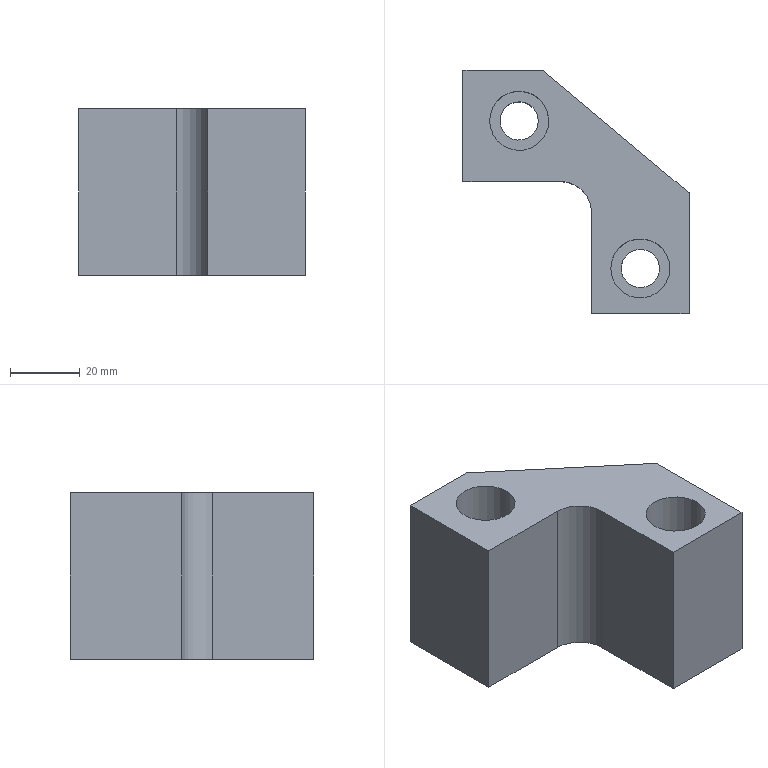Part | STEP file | gslz 2016.10.28-13_id410_x_t | 1 solid | 16 faces | box 65 x 70 x 48 mm | volume 100380 mm3 | plane 11 | cylinder 5 | commonest cylinder face diameters 11 x2 17 x2 18 x1
STEP:
#1=CARTESIAN_POINT('',(0.,0.,0.));
#2=DIRECTION('',(0.,0.,1.));
#3=DIRECTION('',(1.,0.,0.));
#4=AXIS2_PLACEMENT_3D('',#1,#2,#3);
#5=CARTESIAN_POINT('',(-792.811,143.164,0.));
#6=VERTEX_POINT('',#5);
#7=CARTESIAN_POINT('',(-792.811,108.466,0.));
#8=VERTEX_POINT('',#7);
#9=CARTESIAN_POINT('',(-792.811,119.466,0.));
#10=DIRECTION('',(0.,-1.,0.));
#11=VECTOR('',#10,1.);
#12=LINE('',#9,#11);
#13=CARTESIAN_POINT('',(-903.298,257.488,0.));
#14=DIRECTION('',(0.,0.,-1.));
#15=DIRECTION('',(-1.,0.,0.));
#16=AXIS2_PLACEMENT_3D('',#13,#14,#15);
#17=PLANE('',#16);
#18=CARTESIAN_POINT('',(-110.486,-138.022));
#19=DIRECTION('',(0.,-1.));
#20=VECTOR('',#19,1.);
#21=LINE('',#18,#20);
#22=(GEOMETRIC_REPRESENTATION_CONTEXT(2)PARAMETRIC_REPRESENTATION_CONTEXT()REPRESENTATION_CONTEXT('',''));
#23=DEFINITIONAL_REPRESENTATION('',(#21),#22);
#24=PCURVE('',#17,#23);
#25=CARTESIAN_POINT('',(-792.811,119.466,-13.75));
#26=DIRECTION('',(1.,0.,0.));
#27=DIRECTION('',(0.,0.,-1.));
#28=AXIS2_PLACEMENT_3D('',#25,#26,#27);
#29=PLANE('',#28);
#30=CARTESIAN_POINT('',(-13.75,0.));
#31=DIRECTION('',(0.,-1.));
#32=VECTOR('',#31,1.);
#33=LINE('',#30,#32);
#34=(GEOMETRIC_REPRESENTATION_CONTEXT(2)PARAMETRIC_REPRESENTATION_CONTEXT()REPRESENTATION_CONTEXT('',''));
#35=DEFINITIONAL_REPRESENTATION('',(#33),#34);
#36=PCURVE('',#29,#35);
#37=SURFACE_CURVE('',#12,(#24,#36),.PCURVE_S1.);
#38=EDGE_CURVE('',#6,#8,#37,.T.);
#39=ORIENTED_EDGE('',*,*,#38,.F.);
#40=CARTESIAN_POINT('',(-834.883,178.466,0.));
#41=VERTEX_POINT('',#40);
#42=CARTESIAN_POINT('',(-810.301,157.839,0.));
#43=DIRECTION('',(0.766,-0.6428,0.));
#44=VECTOR('',#43,1.);
#45=LINE('',#42,#44);
#46=CARTESIAN_POINT('',(-92.997,-99.649));
#47=DIRECTION('',(-0.766,-0.6428));
#48=VECTOR('',#47,1.);
#49=LINE('',#46,#48);
#50=(GEOMETRIC_REPRESENTATION_CONTEXT(2)PARAMETRIC_REPRESENTATION_CONTEXT()REPRESENTATION_CONTEXT('',''));
#51=DEFINITIONAL_REPRESENTATION('',(#49),#50);
#52=PCURVE('',#17,#51);
#53=CARTESIAN_POINT('',(-810.301,157.839,-13.75));
#54=DIRECTION('',(0.6428,0.766,0.));
#55=DIRECTION('',(0.,0.,1.));
#56=AXIS2_PLACEMENT_3D('',#53,#54,#55);
#57=PLANE('',#56);
#58=CARTESIAN_POINT('',(13.75,0.));
#59=DIRECTION('',(0.,1.));
#60=VECTOR('',#59,1.);
#61=LINE('',#58,#60);
#62=(GEOMETRIC_REPRESENTATION_CONTEXT(2)PARAMETRIC_REPRESENTATION_CONTEXT()REPRESENTATION_CONTEXT('',''));
#63=DEFINITIONAL_REPRESENTATION('',(#61),#62);
#64=PCURVE('',#57,#63);
#65=SURFACE_CURVE('',#45,(#52,#64),.PCURVE_S1.);
#66=EDGE_CURVE('',#41,#6,#65,.T.);
#67=ORIENTED_EDGE('',*,*,#66,.F.);
#68=CARTESIAN_POINT('',(-857.811,178.466,0.));
#69=VERTEX_POINT('',#68);
#70=CARTESIAN_POINT('',(-832.811,178.466,0.));
#71=DIRECTION('',(1.,0.,0.));
#72=VECTOR('',#71,1.);
#73=LINE('',#70,#72);
#74=CARTESIAN_POINT('',(-70.486,-79.022));
#75=DIRECTION('',(-1.,0.));
#76=VECTOR('',#75,1.);
#77=LINE('',#74,#76);
#78=(GEOMETRIC_REPRESENTATION_CONTEXT(2)PARAMETRIC_REPRESENTATION_CONTEXT()REPRESENTATION_CONTEXT('',''));
#79=DEFINITIONAL_REPRESENTATION('',(#77),#78);
#80=PCURVE('',#17,#79);
#81=CARTESIAN_POINT('',(-832.811,178.466,-13.75));
#82=DIRECTION('',(0.,-1.,0.));
#83=DIRECTION('',(0.,0.,-1.));
#84=AXIS2_PLACEMENT_3D('',#81,#82,#83);
#85=PLANE('',#84);
#86=CARTESIAN_POINT('',(-13.75,0.));
#87=DIRECTION('',(0.,1.));
#88=VECTOR('',#87,1.);
#89=LINE('',#86,#88);
#90=(GEOMETRIC_REPRESENTATION_CONTEXT(2)PARAMETRIC_REPRESENTATION_CONTEXT()REPRESENTATION_CONTEXT('',''));
#91=DEFINITIONAL_REPRESENTATION('',(#89),#90);
#92=PCURVE('',#85,#91);
#93=SURFACE_CURVE('',#73,(#80,#92),.PCURVE_S1.);
#94=EDGE_CURVE('',#69,#41,#93,.T.);
#95=ORIENTED_EDGE('',*,*,#94,.F.);
#96=CARTESIAN_POINT('',(-857.811,146.466,0.));
#97=VERTEX_POINT('',#96);
#98=CARTESIAN_POINT('',(-857.811,257.488,0.));
#99=DIRECTION('',(0.,-1.,0.));
#100=VECTOR('',#99,1.);
#101=LINE('',#98,#100);
#102=CARTESIAN_POINT('',(-45.486,0.));
#103=DIRECTION('',(0.,-1.));
#104=VECTOR('',#103,1.);
#105=LINE('',#102,#104);
#106=(GEOMETRIC_REPRESENTATION_CONTEXT(2)PARAMETRIC_REPRESENTATION_CONTEXT()REPRESENTATION_CONTEXT('',''));
#107=DEFINITIONAL_REPRESENTATION('',(#105),#106);
#108=PCURVE('',#17,#107);
#109=CARTESIAN_POINT('',(-857.811,119.466,-13.75));
#110=DIRECTION('',(1.,0.,0.));
#111=DIRECTION('',(0.,0.,-1.));
#112=AXIS2_PLACEMENT_3D('',#109,#110,#111);
#113=PLANE('',#112);
#114=CARTESIAN_POINT('',(-13.75,138.022));
#115=DIRECTION('',(0.,-1.));
#116=VECTOR('',#115,1.);
#117=LINE('',#114,#116);
#118=(GEOMETRIC_REPRESENTATION_CONTEXT(2)PARAMETRIC_REPRESENTATION_CONTEXT()REPRESENTATION_CONTEXT('',''));
#119=DEFINITIONAL_REPRESENTATION('',(#117),#118);
#120=PCURVE('',#113,#119);
#121=SURFACE_CURVE('',#101,(#108,#120),.PCURVE_S1.);
#122=EDGE_CURVE('',#69,#97,#121,.T.);
#123=ORIENTED_EDGE('',*,*,#122,.T.);
#124=CARTESIAN_POINT('',(-829.811,146.466,0.));
#125=VERTEX_POINT('',#124);
#126=CARTESIAN_POINT('',(-832.811,146.466,0.));
#127=DIRECTION('',(-1.,0.,0.));
#128=VECTOR('',#127,1.);
#129=LINE('',#126,#128);
#130=CARTESIAN_POINT('',(-70.486,-111.022));
#131=DIRECTION('',(1.,0.));
#132=VECTOR('',#131,1.);
#133=LINE('',#130,#132);
#134=(GEOMETRIC_REPRESENTATION_CONTEXT(2)PARAMETRIC_REPRESENTATION_CONTEXT()REPRESENTATION_CONTEXT('',''));
#135=DEFINITIONAL_REPRESENTATION('',(#133),#134);
#136=PCURVE('',#17,#135);
#137=CARTESIAN_POINT('',(-832.811,146.466,-13.75));
#138=DIRECTION('',(0.,-1.,0.));
#139=DIRECTION('',(0.,0.,-1.));
#140=AXIS2_PLACEMENT_3D('',#137,#138,#139);
#141=PLANE('',#140);
#142=CARTESIAN_POINT('',(-13.75,0.));
#143=DIRECTION('',(0.,-1.));
#144=VECTOR('',#143,1.);
#145=LINE('',#142,#144);
#146=(GEOMETRIC_REPRESENTATION_CONTEXT(2)PARAMETRIC_REPRESENTATION_CONTEXT()REPRESENTATION_CONTEXT('',''));
#147=DEFINITIONAL_REPRESENTATION('',(#145),#146);
#148=PCURVE('',#141,#147);
#149=SURFACE_CURVE('',#129,(#136,#148),.PCURVE_S1.);
#150=EDGE_CURVE('',#125,#97,#149,.T.);
#151=ORIENTED_EDGE('',*,*,#150,.F.);
#152=CARTESIAN_POINT('',(-820.811,137.466,0.));
#153=VERTEX_POINT('',#152);
#154=CARTESIAN_POINT('',(-829.811,137.466,0.));
#155=DIRECTION('',(0.,0.,-1.));
#156=DIRECTION('',(-1.,0.,0.));
#157=AXIS2_PLACEMENT_3D('',#154,#155,#156);
#158=CIRCLE('',#157,9.);
#159=CARTESIAN_POINT('',(-73.486,-120.022));
#160=DIRECTION('',(1.,0.));
#161=AXIS2_PLACEMENT_2D('',#159,#160);
#162=CIRCLE('',#161,9.);
#163=(GEOMETRIC_REPRESENTATION_CONTEXT(2)PARAMETRIC_REPRESENTATION_CONTEXT()REPRESENTATION_CONTEXT('',''));
#164=DEFINITIONAL_REPRESENTATION('',(#162),#163);
#165=PCURVE('',#17,#164);
#166=CARTESIAN_POINT('',(-829.811,137.466,-13.75));
#167=DIRECTION('',(0.,0.,1.));
#168=DIRECTION('',(1.,0.,0.));
#169=AXIS2_PLACEMENT_3D('',#166,#167,#168);
#170=CYLINDRICAL_SURFACE('',#169,9.);
#171=CARTESIAN_POINT('',(3.142,13.75));
#172=DIRECTION('',(-1.,0.));
#173=VECTOR('',#172,1.);
#174=LINE('',#171,#173);
#175=(GEOMETRIC_REPRESENTATION_CONTEXT(2)PARAMETRIC_REPRESENTATION_CONTEXT()REPRESENTATION_CONTEXT('',''));
#176=DEFINITIONAL_REPRESENTATION('',(#174),#175);
#177=PCURVE('',#170,#176);
#178=SURFACE_CURVE('',#158,(#165,#177),.PCURVE_S1.);
#179=EDGE_CURVE('',#125,#153,#178,.T.);
#180=ORIENTED_EDGE('',*,*,#179,.T.);
#181=CARTESIAN_POINT('',(-820.811,108.466,0.));
#182=VERTEX_POINT('',#181);
#183=CARTESIAN_POINT('',(-820.811,121.466,0.));
#184=DIRECTION('',(0.,-1.,0.));
#185=VECTOR('',#184,1.);
#186=LINE('',#183,#185);
#187=CARTESIAN_POINT('',(-82.486,-136.022));
#188=DIRECTION('',(0.,-1.));
#189=VECTOR('',#188,1.);
#190=LINE('',#187,#189);
#191=(GEOMETRIC_REPRESENTATION_CONTEXT(2)PARAMETRIC_REPRESENTATION_CONTEXT()REPRESENTATION_CONTEXT('',''));
#192=DEFINITIONAL_REPRESENTATION('',(#190),#191);
#193=PCURVE('',#17,#192);
#194=CARTESIAN_POINT('',(-820.811,121.466,-13.75));
#195=DIRECTION('',(1.,0.,0.));
#196=DIRECTION('',(0.,0.,-1.));
#197=AXIS2_PLACEMENT_3D('',#194,#195,#196);
#198=PLANE('',#197);
#199=CARTESIAN_POINT('',(-13.75,0.));
#200=DIRECTION('',(0.,-1.));
#201=VECTOR('',#200,1.);
#202=LINE('',#199,#201);
#203=(GEOMETRIC_REPRESENTATION_CONTEXT(2)PARAMETRIC_REPRESENTATION_CONTEXT()REPRESENTATION_CONTEXT('',''));
#204=DEFINITIONAL_REPRESENTATION('',(#202),#203);
#205=PCURVE('',#198,#204);
#206=SURFACE_CURVE('',#186,(#193,#205),.PCURVE_S1.);
#207=EDGE_CURVE('',#153,#182,#206,.T.);
#208=ORIENTED_EDGE('',*,*,#207,.T.);
#209=CARTESIAN_POINT('',(-832.811,108.466,0.));
#210=DIRECTION('',(-1.,0.,0.));
#211=VECTOR('',#210,1.);
#212=LINE('',#209,#211);
#213=CARTESIAN_POINT('',(-70.486,-149.022));
#214=DIRECTION('',(1.,0.));
#215=VECTOR('',#214,1.);
#216=LINE('',#213,#215);
#217=(GEOMETRIC_REPRESENTATION_CONTEXT(2)PARAMETRIC_REPRESENTATION_CONTEXT()REPRESENTATION_CONTEXT('',''));
#218=DEFINITIONAL_REPRESENTATION('',(#216),#217);
#219=PCURVE('',#17,#218);
#220=CARTESIAN_POINT('',(-832.811,108.466,-13.75));
#221=DIRECTION('',(0.,-1.,0.));
#222=DIRECTION('',(0.,0.,-1.));
#223=AXIS2_PLACEMENT_3D('',#220,#221,#222);
#224=PLANE('',#223);
#225=CARTESIAN_POINT('',(-13.75,0.));
#226=DIRECTION('',(0.,-1.));
#227=VECTOR('',#226,1.);
#228=LINE('',#225,#227);
#229=(GEOMETRIC_REPRESENTATION_CONTEXT(2)PARAMETRIC_REPRESENTATION_CONTEXT()REPRESENTATION_CONTEXT('',''));
#230=DEFINITIONAL_REPRESENTATION('',(#228),#229);
#231=PCURVE('',#224,#230);
#232=SURFACE_CURVE('',#212,(#219,#231),.PCURVE_S1.);
#233=EDGE_CURVE('',#8,#182,#232,.T.);
#234=ORIENTED_EDGE('',*,*,#233,.F.);
#235=EDGE_LOOP('',(#39,#67,#95,#123,#151,#180,#208,#234));
#236=FACE_BOUND('',#235,.T.);
#237=CARTESIAN_POINT('',(-815.311,121.466,0.));
#238=VERTEX_POINT('',#237);
#239=CARTESIAN_POINT('',(-806.811,121.466,0.));
#240=DIRECTION('',(0.,0.,-1.));
#241=DIRECTION('',(-1.,0.,0.));
#242=AXIS2_PLACEMENT_3D('',#239,#240,#241);
#243=CIRCLE('',#242,8.5);
#244=CARTESIAN_POINT('',(-96.486,-136.022));
#245=DIRECTION('',(1.,0.));
#246=AXIS2_PLACEMENT_2D('',#244,#245);
#247=CIRCLE('',#246,8.5);
#248=(GEOMETRIC_REPRESENTATION_CONTEXT(2)PARAMETRIC_REPRESENTATION_CONTEXT()REPRESENTATION_CONTEXT('',''));
#249=DEFINITIONAL_REPRESENTATION('',(#247),#248);
#250=PCURVE('',#17,#249);
#251=CARTESIAN_POINT('',(-806.811,121.466,0.));
#252=DIRECTION('',(0.,0.,-1.));
#253=DIRECTION('',(-1.,0.,0.));
#254=AXIS2_PLACEMENT_3D('',#251,#252,#253);
#255=CYLINDRICAL_SURFACE('',#254,8.5);
#256=CARTESIAN_POINT('',(0.,0.));
#257=DIRECTION('',(1.,0.));
#258=VECTOR('',#257,1.);
#259=LINE('',#256,#258);
#260=(GEOMETRIC_REPRESENTATION_CONTEXT(2)PARAMETRIC_REPRESENTATION_CONTEXT()REPRESENTATION_CONTEXT('',''));
#261=DEFINITIONAL_REPRESENTATION('',(#259),#260);
#262=PCURVE('',#255,#261);
#263=SURFACE_CURVE('',#243,(#250,#262),.PCURVE_S1.);
#264=EDGE_CURVE('',#238,#238,#263,.T.);
#265=ORIENTED_EDGE('',*,*,#264,.T.);
#266=EDGE_LOOP('',(#265));
#267=FACE_BOUND('',#266,.T.);
#268=CARTESIAN_POINT('',(-848.157,169.355,0.));
#269=VERTEX_POINT('',#268);
#270=CARTESIAN_POINT('',(-841.646,163.891,0.));
#271=DIRECTION('',(0.,0.,-1.));
#272=DIRECTION('',(-0.766,0.6428,0.));
#273=AXIS2_PLACEMENT_3D('',#270,#271,#272);
#274=CIRCLE('',#273,8.5);
#275=CARTESIAN_POINT('',(-61.652,-93.597));
#276=DIRECTION('',(0.766,0.6428));
#277=AXIS2_PLACEMENT_2D('',#275,#276);
#278=CIRCLE('',#277,8.5);
#279=(GEOMETRIC_REPRESENTATION_CONTEXT(2)PARAMETRIC_REPRESENTATION_CONTEXT()REPRESENTATION_CONTEXT('',''));
#280=DEFINITIONAL_REPRESENTATION('',(#278),#279);
#281=PCURVE('',#17,#280);
#282=CARTESIAN_POINT('',(-841.646,163.891,0.));
#283=DIRECTION('',(0.,0.,-1.));
#284=DIRECTION('',(-0.766,0.6428,0.));
#285=AXIS2_PLACEMENT_3D('',#282,#283,#284);
#286=CYLINDRICAL_SURFACE('',#285,8.5);
#287=CARTESIAN_POINT('',(0.,0.));
#288=DIRECTION('',(1.,0.));
#289=VECTOR('',#288,1.);
#290=LINE('',#287,#289);
#291=(GEOMETRIC_REPRESENTATION_CONTEXT(2)PARAMETRIC_REPRESENTATION_CONTEXT()REPRESENTATION_CONTEXT('',''));
#292=DEFINITIONAL_REPRESENTATION('',(#290),#291);
#293=PCURVE('',#286,#292);
#294=SURFACE_CURVE('',#274,(#281,#293),.PCURVE_S1.);
#295=EDGE_CURVE('',#269,#269,#294,.T.);
#296=ORIENTED_EDGE('',*,*,#295,.T.);
#297=EDGE_LOOP('',(#296));
#298=FACE_BOUND('',#297,.T.);
#299=ADVANCED_FACE('',(#236,#267,#298),#17,.F.);
#300=CARTESIAN_POINT('',(-820.811,108.466,-48.));
#301=VERTEX_POINT('',#300);
#302=CARTESIAN_POINT('',(-820.811,108.466,-13.75));
#303=DIRECTION('',(0.,0.,1.));
#304=VECTOR('',#303,1.);
#305=LINE('',#302,#304);
#306=CARTESIAN_POINT('',(0.,12.));
#307=DIRECTION('',(-1.,0.));
#308=VECTOR('',#307,1.);
#309=LINE('',#306,#308);
#310=(GEOMETRIC_REPRESENTATION_CONTEXT(2)PARAMETRIC_REPRESENTATION_CONTEXT()REPRESENTATION_CONTEXT('',''));
#311=DEFINITIONAL_REPRESENTATION('',(#309),#310);
#312=PCURVE('',#224,#311);
#313=CARTESIAN_POINT('',(0.,-13.));
#314=DIRECTION('',(-1.,0.));
#315=VECTOR('',#314,1.);
#316=LINE('',#313,#315);
#317=(GEOMETRIC_REPRESENTATION_CONTEXT(2)PARAMETRIC_REPRESENTATION_CONTEXT()REPRESENTATION_CONTEXT('',''));
#318=DEFINITIONAL_REPRESENTATION('',(#316),#317);
#319=PCURVE('',#198,#318);
#320=SURFACE_CURVE('',#305,(#312,#319),.PCURVE_S1.);
#321=EDGE_CURVE('',#301,#182,#320,.T.);
#322=ORIENTED_EDGE('',*,*,#321,.F.);
#323=CARTESIAN_POINT('',(-792.811,108.466,-48.));
#324=VERTEX_POINT('',#323);
#325=CARTESIAN_POINT('',(-832.811,108.466,-48.));
#326=DIRECTION('',(1.,0.,0.));
#327=VECTOR('',#326,1.);
#328=LINE('',#325,#327);
#329=CARTESIAN_POINT('',(34.25,0.));
#330=DIRECTION('',(0.,1.));
#331=VECTOR('',#330,1.);
#332=LINE('',#329,#331);
#333=(GEOMETRIC_REPRESENTATION_CONTEXT(2)PARAMETRIC_REPRESENTATION_CONTEXT()REPRESENTATION_CONTEXT('',''));
#334=DEFINITIONAL_REPRESENTATION('',(#332),#333);
#335=PCURVE('',#224,#334);
#336=CARTESIAN_POINT('',(-903.298,257.488,-48.));
#337=DIRECTION('',(0.,0.,-1.));
#338=DIRECTION('',(-1.,0.,0.));
#339=AXIS2_PLACEMENT_3D('',#336,#337,#338);
#340=PLANE('',#339);
#341=CARTESIAN_POINT('',(-70.486,-149.022));
#342=DIRECTION('',(-1.,0.));
#343=VECTOR('',#342,1.);
#344=LINE('',#341,#343);
#345=(GEOMETRIC_REPRESENTATION_CONTEXT(2)PARAMETRIC_REPRESENTATION_CONTEXT()REPRESENTATION_CONTEXT('',''));
#346=DEFINITIONAL_REPRESENTATION('',(#344),#345);
#347=PCURVE('',#340,#346);
#348=SURFACE_CURVE('',#328,(#335,#347),.PCURVE_S1.);
#349=EDGE_CURVE('',#301,#324,#348,.T.);
#350=ORIENTED_EDGE('',*,*,#349,.T.);
#351=CARTESIAN_POINT('',(-792.811,108.466,-13.75));
#352=DIRECTION('',(0.,0.,1.));
#353=VECTOR('',#352,1.);
#354=LINE('',#351,#353);
#355=CARTESIAN_POINT('',(0.,40.));
#356=DIRECTION('',(-1.,0.));
#357=VECTOR('',#356,1.);
#358=LINE('',#355,#357);
#359=(GEOMETRIC_REPRESENTATION_CONTEXT(2)PARAMETRIC_REPRESENTATION_CONTEXT()REPRESENTATION_CONTEXT('',''));
#360=DEFINITIONAL_REPRESENTATION('',(#358),#359);
#361=PCURVE('',#224,#360);
#362=CARTESIAN_POINT('',(0.,-11.));
#363=DIRECTION('',(-1.,0.));
#364=VECTOR('',#363,1.);
#365=LINE('',#362,#364);
#366=(GEOMETRIC_REPRESENTATION_CONTEXT(2)PARAMETRIC_REPRESENTATION_CONTEXT()REPRESENTATION_CONTEXT('',''));
#367=DEFINITIONAL_REPRESENTATION('',(#365),#366);
#368=PCURVE('',#29,#367);
#369=SURFACE_CURVE('',#354,(#361,#368),.PCURVE_S1.);
#370=EDGE_CURVE('',#324,#8,#369,.T.);
#371=ORIENTED_EDGE('',*,*,#370,.T.);
#372=ORIENTED_EDGE('',*,*,#233,.T.);
#373=EDGE_LOOP('',(#322,#350,#371,#372));
#374=FACE_BOUND('',#373,.T.);
#375=ADVANCED_FACE('',(#374),#224,.T.);
#376=CARTESIAN_POINT('',(-792.811,143.164,-48.));
#377=VERTEX_POINT('',#376);
#378=CARTESIAN_POINT('',(-834.883,178.466,-48.));
#379=VERTEX_POINT('',#378);
#380=CARTESIAN_POINT('',(-810.301,157.839,-48.));
#381=DIRECTION('',(-0.766,0.6428,0.));
#382=VECTOR('',#381,1.);
#383=LINE('',#380,#382);
#384=CARTESIAN_POINT('',(-92.997,-99.649));
#385=DIRECTION('',(0.766,0.6428));
#386=VECTOR('',#385,1.);
#387=LINE('',#384,#386);
#388=(GEOMETRIC_REPRESENTATION_CONTEXT(2)PARAMETRIC_REPRESENTATION_CONTEXT()REPRESENTATION_CONTEXT('',''));
#389=DEFINITIONAL_REPRESENTATION('',(#387),#388);
#390=PCURVE('',#340,#389);
#391=CARTESIAN_POINT('',(-34.25,0.));
#392=DIRECTION('',(0.,-1.));
#393=VECTOR('',#392,1.);
#394=LINE('',#391,#393);
#395=(GEOMETRIC_REPRESENTATION_CONTEXT(2)PARAMETRIC_REPRESENTATION_CONTEXT()REPRESENTATION_CONTEXT('',''));
#396=DEFINITIONAL_REPRESENTATION('',(#394),#395);
#397=PCURVE('',#57,#396);
#398=SURFACE_CURVE('',#383,(#390,#397),.PCURVE_S1.);
#399=EDGE_CURVE('',#377,#379,#398,.T.);
#400=ORIENTED_EDGE('',*,*,#399,.F.);
#401=CARTESIAN_POINT('',(-792.811,119.466,-48.));
#402=DIRECTION('',(0.,1.,0.));
#403=VECTOR('',#402,1.);
#404=LINE('',#401,#403);
#405=CARTESIAN_POINT('',(-110.486,-138.022));
#406=DIRECTION('',(0.,1.));
#407=VECTOR('',#406,1.);
#408=LINE('',#405,#407);
#409=(GEOMETRIC_REPRESENTATION_CONTEXT(2)PARAMETRIC_REPRESENTATION_CONTEXT()REPRESENTATION_CONTEXT('',''));
#410=DEFINITIONAL_REPRESENTATION('',(#408),#409);
#411=PCURVE('',#340,#410);
#412=CARTESIAN_POINT('',(34.25,0.));
#413=DIRECTION('',(0.,1.));
#414=VECTOR('',#413,1.);
#415=LINE('',#412,#414);
#416=(GEOMETRIC_REPRESENTATION_CONTEXT(2)PARAMETRIC_REPRESENTATION_CONTEXT()REPRESENTATION_CONTEXT('',''));
#417=DEFINITIONAL_REPRESENTATION('',(#415),#416);
#418=PCURVE('',#29,#417);
#419=SURFACE_CURVE('',#404,(#411,#418),.PCURVE_S1.);
#420=EDGE_CURVE('',#324,#377,#419,.T.);
#421=ORIENTED_EDGE('',*,*,#420,.F.);
#422=ORIENTED_EDGE('',*,*,#349,.F.);
#423=CARTESIAN_POINT('',(-820.811,137.466,-48.));
#424=VERTEX_POINT('',#423);
#425=CARTESIAN_POINT('',(-820.811,259.488,-48.));
#426=DIRECTION('',(0.,-1.,0.));
#427=VECTOR('',#426,1.);
#428=LINE('',#425,#427);
#429=CARTESIAN_POINT('',(-82.486,2.));
#430=DIRECTION('',(0.,-1.));
#431=VECTOR('',#430,1.);
#432=LINE('',#429,#431);
#433=(GEOMETRIC_REPRESENTATION_CONTEXT(2)PARAMETRIC_REPRESENTATION_CONTEXT()REPRESENTATION_CONTEXT('',''));
#434=DEFINITIONAL_REPRESENTATION('',(#432),#433);
#435=PCURVE('',#340,#434);
#436=CARTESIAN_POINT('',(34.25,138.022));
#437=DIRECTION('',(0.,-1.));
#438=VECTOR('',#437,1.);
#439=LINE('',#436,#438);
#440=(GEOMETRIC_REPRESENTATION_CONTEXT(2)PARAMETRIC_REPRESENTATION_CONTEXT()REPRESENTATION_CONTEXT('',''));
#441=DEFINITIONAL_REPRESENTATION('',(#439),#440);
#442=PCURVE('',#198,#441);
#443=SURFACE_CURVE('',#428,(#435,#442),.PCURVE_S1.);
#444=EDGE_CURVE('',#424,#301,#443,.T.);
#445=ORIENTED_EDGE('',*,*,#444,.F.);
#446=CARTESIAN_POINT('',(-829.811,146.466,-48.));
#447=VERTEX_POINT('',#446);
#448=CARTESIAN_POINT('',(-829.811,137.466,-48.));
#449=DIRECTION('',(0.,0.,1.));
#450=DIRECTION('',(-1.,0.,0.));
#451=AXIS2_PLACEMENT_3D('',#448,#449,#450);
#452=CIRCLE('',#451,9.);
#453=CARTESIAN_POINT('',(-64.486,-120.022));
#454=CARTESIAN_POINT('',(-64.486,-135.611));
#455=CARTESIAN_POINT('',(-77.986,-127.816));
#456=CARTESIAN_POINT('',(-91.486,-120.022));
#457=CARTESIAN_POINT('',(-77.986,-112.228));
#458=CARTESIAN_POINT('',(-64.486,-104.434));
#459=CARTESIAN_POINT('',(-64.486,-120.022));
#460=(BOUNDED_CURVE()B_SPLINE_CURVE(2,(#453,#454,#455,#456,#457,#458,#459),.UNSPECIFIED.,.T.,.F.)B_SPLINE_CURVE_WITH_KNOTS((1,2,2,2,2,1),(-2.094,0.,2.094,4.189,6.283,8.378),.UNSPECIFIED.)CURVE()GEOMETRIC_REPRESENTATION_ITEM()RATIONAL_B_SPLINE_CURVE((1.,0.5,1.,0.5,1.,0.5,1.))REPRESENTATION_ITEM(''));
#461=(GEOMETRIC_REPRESENTATION_CONTEXT(2)PARAMETRIC_REPRESENTATION_CONTEXT()REPRESENTATION_CONTEXT('',''));
#462=DEFINITIONAL_REPRESENTATION('',(#460),#461);
#463=PCURVE('',#340,#462);
#464=CARTESIAN_POINT('',(-3.142,-34.25));
#465=DIRECTION('',(1.,0.));
#466=VECTOR('',#465,1.);
#467=LINE('',#464,#466);
#468=(GEOMETRIC_REPRESENTATION_CONTEXT(2)PARAMETRIC_REPRESENTATION_CONTEXT()REPRESENTATION_CONTEXT('',''));
#469=DEFINITIONAL_REPRESENTATION('',(#467),#468);
#470=PCURVE('',#170,#469);
#471=SURFACE_CURVE('',#452,(#463,#470),.PCURVE_S1.);
#472=EDGE_CURVE('',#424,#447,#471,.T.);
#473=ORIENTED_EDGE('',*,*,#472,.T.);
#474=CARTESIAN_POINT('',(-857.811,146.466,-48.));
#475=VERTEX_POINT('',#474);
#476=CARTESIAN_POINT('',(-832.811,146.466,-48.));
#477=DIRECTION('',(1.,0.,0.));
#478=VECTOR('',#477,1.);
#479=LINE('',#476,#478);
#480=CARTESIAN_POINT('',(-70.486,-111.022));
#481=DIRECTION('',(-1.,0.));
#482=VECTOR('',#481,1.);
#483=LINE('',#480,#482);
#484=(GEOMETRIC_REPRESENTATION_CONTEXT(2)PARAMETRIC_REPRESENTATION_CONTEXT()REPRESENTATION_CONTEXT('',''));
#485=DEFINITIONAL_REPRESENTATION('',(#483),#484);
#486=PCURVE('',#340,#485);
#487=CARTESIAN_POINT('',(34.25,0.));
#488=DIRECTION('',(0.,1.));
#489=VECTOR('',#488,1.);
#490=LINE('',#487,#489);
#491=(GEOMETRIC_REPRESENTATION_CONTEXT(2)PARAMETRIC_REPRESENTATION_CONTEXT()REPRESENTATION_CONTEXT('',''));
#492=DEFINITIONAL_REPRESENTATION('',(#490),#491);
#493=PCURVE('',#141,#492);
#494=SURFACE_CURVE('',#479,(#486,#493),.PCURVE_S1.);
#495=EDGE_CURVE('',#475,#447,#494,.T.);
#496=ORIENTED_EDGE('',*,*,#495,.F.);
#497=CARTESIAN_POINT('',(-857.811,178.466,-48.));
#498=VERTEX_POINT('',#497);
#499=CARTESIAN_POINT('',(-857.811,257.488,-48.));
#500=DIRECTION('',(0.,1.,0.));
#501=VECTOR('',#500,1.);
#502=LINE('',#499,#501);
#503=CARTESIAN_POINT('',(-45.486,0.));
#504=DIRECTION('',(0.,1.));
#505=VECTOR('',#504,1.);
#506=LINE('',#503,#505);
#507=(GEOMETRIC_REPRESENTATION_CONTEXT(2)PARAMETRIC_REPRESENTATION_CONTEXT()REPRESENTATION_CONTEXT('',''));
#508=DEFINITIONAL_REPRESENTATION('',(#506),#507);
#509=PCURVE('',#340,#508);
#510=CARTESIAN_POINT('',(34.25,138.022));
#511=DIRECTION('',(0.,1.));
#512=VECTOR('',#511,1.);
#513=LINE('',#510,#512);
#514=(GEOMETRIC_REPRESENTATION_CONTEXT(2)PARAMETRIC_REPRESENTATION_CONTEXT()REPRESENTATION_CONTEXT('',''));
#515=DEFINITIONAL_REPRESENTATION('',(#513),#514);
#516=PCURVE('',#113,#515);
#517=SURFACE_CURVE('',#502,(#509,#516),.PCURVE_S1.);
#518=EDGE_CURVE('',#475,#498,#517,.T.);
#519=ORIENTED_EDGE('',*,*,#518,.T.);
#520=CARTESIAN_POINT('',(-832.811,178.466,-48.));
#521=DIRECTION('',(-1.,0.,0.));
#522=VECTOR('',#521,1.);
#523=LINE('',#520,#522);
#524=CARTESIAN_POINT('',(-70.486,-79.022));
#525=DIRECTION('',(1.,0.));
#526=VECTOR('',#525,1.);
#527=LINE('',#524,#526);
#528=(GEOMETRIC_REPRESENTATION_CONTEXT(2)PARAMETRIC_REPRESENTATION_CONTEXT()REPRESENTATION_CONTEXT('',''));
#529=DEFINITIONAL_REPRESENTATION('',(#527),#528);
#530=PCURVE('',#340,#529);
#531=CARTESIAN_POINT('',(34.25,0.));
#532=DIRECTION('',(0.,-1.));
#533=VECTOR('',#532,1.);
#534=LINE('',#531,#533);
#535=(GEOMETRIC_REPRESENTATION_CONTEXT(2)PARAMETRIC_REPRESENTATION_CONTEXT()REPRESENTATION_CONTEXT('',''));
#536=DEFINITIONAL_REPRESENTATION('',(#534),#535);
#537=PCURVE('',#85,#536);
#538=SURFACE_CURVE('',#523,(#530,#537),.PCURVE_S1.);
#539=EDGE_CURVE('',#379,#498,#538,.T.);
#540=ORIENTED_EDGE('',*,*,#539,.F.);
#541=EDGE_LOOP('',(#400,#421,#422,#445,#473,#496,#519,#540));
#542=FACE_BOUND('',#541,.T.);
#543=CARTESIAN_POINT('',(-812.311,121.466,-48.));
#544=VERTEX_POINT('',#543);
#545=CARTESIAN_POINT('',(-806.811,121.466,-48.));
#546=DIRECTION('',(0.,0.,-1.));
#547=DIRECTION('',(-1.,0.,0.));
#548=AXIS2_PLACEMENT_3D('',#545,#546,#547);
#549=CIRCLE('',#548,5.5);
#550=CARTESIAN_POINT('',(-96.486,-136.022));
#551=DIRECTION('',(1.,0.));
#552=AXIS2_PLACEMENT_2D('',#550,#551);
#553=CIRCLE('',#552,5.5);
#554=(GEOMETRIC_REPRESENTATION_CONTEXT(2)PARAMETRIC_REPRESENTATION_CONTEXT()REPRESENTATION_CONTEXT('',''));
#555=DEFINITIONAL_REPRESENTATION('',(#553),#554);
#556=PCURVE('',#340,#555);
#557=CARTESIAN_POINT('',(-806.811,121.466,-150.));
#558=DIRECTION('',(0.,0.,-1.));
#559=DIRECTION('',(-1.,0.,0.));
#560=AXIS2_PLACEMENT_3D('',#557,#558,#559);
#561=CYLINDRICAL_SURFACE('',#560,5.5);
#562=CARTESIAN_POINT('',(0.,-102.));
#563=DIRECTION('',(1.,0.));
#564=VECTOR('',#563,1.);
#565=LINE('',#562,#564);
#566=(GEOMETRIC_REPRESENTATION_CONTEXT(2)PARAMETRIC_REPRESENTATION_CONTEXT()REPRESENTATION_CONTEXT('',''));
#567=DEFINITIONAL_REPRESENTATION('',(#565),#566);
#568=PCURVE('',#561,#567);
#569=SURFACE_CURVE('',#549,(#556,#568),.PCURVE_S1.);
#570=EDGE_CURVE('',#544,#544,#569,.T.);
#571=ORIENTED_EDGE('',*,*,#570,.F.);
#572=EDGE_LOOP('',(#571));
#573=FACE_BOUND('',#572,.T.);
#574=CARTESIAN_POINT('',(-845.859,167.426,-48.));
#575=VERTEX_POINT('',#574);
#576=CARTESIAN_POINT('',(-841.646,163.891,-48.));
#577=DIRECTION('',(0.,0.,-1.));
#578=DIRECTION('',(-0.766,0.6428,0.));
#579=AXIS2_PLACEMENT_3D('',#576,#577,#578);
#580=CIRCLE('',#579,5.5);
#581=CARTESIAN_POINT('',(-61.652,-93.597));
#582=DIRECTION('',(0.766,0.6428));
#583=AXIS2_PLACEMENT_2D('',#581,#582);
#584=CIRCLE('',#583,5.5);
#585=(GEOMETRIC_REPRESENTATION_CONTEXT(2)PARAMETRIC_REPRESENTATION_CONTEXT()REPRESENTATION_CONTEXT('',''));
#586=DEFINITIONAL_REPRESENTATION('',(#584),#585);
#587=PCURVE('',#340,#586);
#588=CARTESIAN_POINT('',(-841.646,163.891,-150.));
#589=DIRECTION('',(0.,0.,-1.));
#590=DIRECTION('',(-0.766,0.6428,0.));
#591=AXIS2_PLACEMENT_3D('',#588,#589,#590);
#592=CYLINDRICAL_SURFACE('',#591,5.5);
#593=CARTESIAN_POINT('',(0.,-102.));
#594=DIRECTION('',(1.,0.));
#595=VECTOR('',#594,1.);
#596=LINE('',#593,#595);
#597=(GEOMETRIC_REPRESENTATION_CONTEXT(2)PARAMETRIC_REPRESENTATION_CONTEXT()REPRESENTATION_CONTEXT('',''));
#598=DEFINITIONAL_REPRESENTATION('',(#596),#597);
#599=PCURVE('',#592,#598);
#600=SURFACE_CURVE('',#580,(#587,#599),.PCURVE_S1.);
#601=EDGE_CURVE('',#575,#575,#600,.T.);
#602=ORIENTED_EDGE('',*,*,#601,.F.);
#603=EDGE_LOOP('',(#602));
#604=FACE_BOUND('',#603,.T.);
#605=ADVANCED_FACE('',(#542,#573,#604),#340,.T.);
#606=ORIENTED_EDGE('',*,*,#420,.T.);
#607=CARTESIAN_POINT('',(-792.811,143.164,-13.75));
#608=DIRECTION('',(0.,0.,1.));
#609=VECTOR('',#608,1.);
#610=LINE('',#607,#609);
#611=CARTESIAN_POINT('',(0.,23.698));
#612=DIRECTION('',(-1.,0.));
#613=VECTOR('',#612,1.);
#614=LINE('',#611,#613);
#615=(GEOMETRIC_REPRESENTATION_CONTEXT(2)PARAMETRIC_REPRESENTATION_CONTEXT()REPRESENTATION_CONTEXT('',''));
#616=DEFINITIONAL_REPRESENTATION('',(#614),#615);
#617=PCURVE('',#29,#616);
#618=CARTESIAN_POINT('',(0.,22.831));
#619=DIRECTION('',(1.,0.));
#620=VECTOR('',#619,1.);
#621=LINE('',#618,#620);
#622=(GEOMETRIC_REPRESENTATION_CONTEXT(2)PARAMETRIC_REPRESENTATION_CONTEXT()REPRESENTATION_CONTEXT('',''));
#623=DEFINITIONAL_REPRESENTATION('',(#621),#622);
#624=PCURVE('',#57,#623);
#625=SURFACE_CURVE('',#610,(#617,#624),.PCURVE_S1.);
#626=EDGE_CURVE('',#377,#6,#625,.T.);
#627=ORIENTED_EDGE('',*,*,#626,.T.);
#628=ORIENTED_EDGE('',*,*,#38,.T.);
#629=ORIENTED_EDGE('',*,*,#370,.F.);
#630=EDGE_LOOP('',(#606,#627,#628,#629));
#631=FACE_BOUND('',#630,.T.);
#632=ADVANCED_FACE('',(#631),#29,.T.);
#633=ORIENTED_EDGE('',*,*,#570,.F.);
#634=CARTESIAN_POINT('',(-812.311,121.466,-25.));
#635=VERTEX_POINT('',#634);
#636=CARTESIAN_POINT('',(-812.311,121.466,-25.));
#637=CARTESIAN_POINT('',(-812.311,121.466,-48.));
#638=B_SPLINE_CURVE_WITH_KNOTS('',1,(#636,#637),.UNSPECIFIED.,.F.,.F.,(2,2),(-125.,-102.),.PIECEWISE_BEZIER_KNOTS.);
#639=CARTESIAN_POINT('',(0.,0.));
#640=DIRECTION('',(0.,1.));
#641=VECTOR('',#640,1.);
#642=LINE('',#639,#641);
#643=(GEOMETRIC_REPRESENTATION_CONTEXT(2)PARAMETRIC_REPRESENTATION_CONTEXT()REPRESENTATION_CONTEXT('',''));
#644=DEFINITIONAL_REPRESENTATION('',(#642),#643);
#645=PCURVE('',#561,#644);
#646=CARTESIAN_POINT('',(6.283,0.));
#647=DIRECTION('',(0.,1.));
#648=VECTOR('',#647,1.);
#649=LINE('',#646,#648);
#650=(GEOMETRIC_REPRESENTATION_CONTEXT(2)PARAMETRIC_REPRESENTATION_CONTEXT()REPRESENTATION_CONTEXT('',''));
#651=DEFINITIONAL_REPRESENTATION('',(#649),#650);
#652=PCURVE('',#561,#651);
#653=SEAM_CURVE('',#638,(#645,#652),.PCURVE_S1.);
#654=EDGE_CURVE('',#635,#544,#653,.T.);
#655=ORIENTED_EDGE('',*,*,#654,.F.);
#656=CARTESIAN_POINT('',(-806.811,121.466,-25.));
#657=DIRECTION('',(0.,0.,1.));
#658=DIRECTION('',(-1.,0.,0.));
#659=AXIS2_PLACEMENT_3D('',#656,#657,#658);
#660=CIRCLE('',#659,5.5);
#661=CARTESIAN_POINT('',(6.283,-125.));
#662=DIRECTION('',(-1.,0.));
#663=VECTOR('',#662,1.);
#664=LINE('',#661,#663);
#665=(GEOMETRIC_REPRESENTATION_CONTEXT(2)PARAMETRIC_REPRESENTATION_CONTEXT()REPRESENTATION_CONTEXT('',''));
#666=DEFINITIONAL_REPRESENTATION('',(#664),#665);
#667=PCURVE('',#561,#666);
#668=CARTESIAN_POINT('',(-806.811,121.466,-25.));
#669=DIRECTION('',(0.,0.,-1.));
#670=DIRECTION('',(-1.,0.,0.));
#671=AXIS2_PLACEMENT_3D('',#668,#669,#670);
#672=PLANE('',#671);
#673=CARTESIAN_POINT('',(5.5,0.));
#674=CARTESIAN_POINT('',(5.5,-9.526));
#675=CARTESIAN_POINT('',(-2.75,-4.763));
#676=CARTESIAN_POINT('',(-11.,0.));
#677=CARTESIAN_POINT('',(-2.75,4.763));
#678=CARTESIAN_POINT('',(5.5,9.526));
#679=CARTESIAN_POINT('',(5.5,0.));
#680=(BOUNDED_CURVE()B_SPLINE_CURVE(2,(#673,#674,#675,#676,#677,#678,#679),.UNSPECIFIED.,.T.,.F.)B_SPLINE_CURVE_WITH_KNOTS((1,2,2,2,2,1),(-2.094,0.,2.094,4.189,6.283,8.378),.UNSPECIFIED.)CURVE()GEOMETRIC_REPRESENTATION_ITEM()RATIONAL_B_SPLINE_CURVE((1.,0.5,1.,0.5,1.,0.5,1.))REPRESENTATION_ITEM(''));
#681=(GEOMETRIC_REPRESENTATION_CONTEXT(2)PARAMETRIC_REPRESENTATION_CONTEXT()REPRESENTATION_CONTEXT('',''));
#682=DEFINITIONAL_REPRESENTATION('',(#680),#681);
#683=PCURVE('',#672,#682);
#684=SURFACE_CURVE('',#660,(#667,#683),.PCURVE_S1.);
#685=EDGE_CURVE('',#635,#635,#684,.T.);
#686=ORIENTED_EDGE('',*,*,#685,.F.);
#687=ORIENTED_EDGE('',*,*,#654,.T.);
#688=EDGE_LOOP('',(#633,#655,#686,#687));
#689=FACE_BOUND('',#688,.F.);
#690=ADVANCED_FACE('',(#689),#561,.F.);
#691=ORIENTED_EDGE('',*,*,#685,.F.);
#692=EDGE_LOOP('',(#691));
#693=FACE_BOUND('',#692,.T.);
#694=CARTESIAN_POINT('',(-815.311,121.466,-25.));
#695=VERTEX_POINT('',#694);
#696=CARTESIAN_POINT('',(-806.811,121.466,-25.));
#697=DIRECTION('',(0.,0.,1.));
#698=DIRECTION('',(-1.,0.,0.));
#699=AXIS2_PLACEMENT_3D('',#696,#697,#698);
#700=CIRCLE('',#699,8.5);
#701=CARTESIAN_POINT('',(8.5,0.));
#702=CARTESIAN_POINT('',(8.5,-14.722));
#703=CARTESIAN_POINT('',(-4.25,-7.361));
#704=CARTESIAN_POINT('',(-17.,0.));
#705=CARTESIAN_POINT('',(-4.25,7.361));
#706=CARTESIAN_POINT('',(8.5,14.722));
#707=CARTESIAN_POINT('',(8.5,0.));
#708=(BOUNDED_CURVE()B_SPLINE_CURVE(2,(#701,#702,#703,#704,#705,#706,#707),.UNSPECIFIED.,.T.,.F.)B_SPLINE_CURVE_WITH_KNOTS((1,2,2,2,2,1),(-2.094,0.,2.094,4.189,6.283,8.378),.UNSPECIFIED.)CURVE()GEOMETRIC_REPRESENTATION_ITEM()RATIONAL_B_SPLINE_CURVE((1.,0.5,1.,0.5,1.,0.5,1.))REPRESENTATION_ITEM(''));
#709=(GEOMETRIC_REPRESENTATION_CONTEXT(2)PARAMETRIC_REPRESENTATION_CONTEXT()REPRESENTATION_CONTEXT('',''));
#710=DEFINITIONAL_REPRESENTATION('',(#708),#709);
#711=PCURVE('',#672,#710);
#712=CARTESIAN_POINT('',(6.283,25.));
#713=DIRECTION('',(-1.,0.));
#714=VECTOR('',#713,1.);
#715=LINE('',#712,#714);
#716=(GEOMETRIC_REPRESENTATION_CONTEXT(2)PARAMETRIC_REPRESENTATION_CONTEXT()REPRESENTATION_CONTEXT('',''));
#717=DEFINITIONAL_REPRESENTATION('',(#715),#716);
#718=PCURVE('',#255,#717);
#719=SURFACE_CURVE('',#700,(#711,#718),.PCURVE_S1.);
#720=EDGE_CURVE('',#695,#695,#719,.T.);
#721=ORIENTED_EDGE('',*,*,#720,.T.);
#722=EDGE_LOOP('',(#721));
#723=FACE_BOUND('',#722,.T.);
#724=ADVANCED_FACE('',(#693,#723),#672,.F.);
#725=ORIENTED_EDGE('',*,*,#720,.T.);
#726=CARTESIAN_POINT('',(-815.311,121.466,0.));
#727=CARTESIAN_POINT('',(-815.311,121.466,-25.));
#728=B_SPLINE_CURVE_WITH_KNOTS('',1,(#726,#727),.UNSPECIFIED.,.F.,.F.,(2,2),(0.,25.),.PIECEWISE_BEZIER_KNOTS.);
#729=CARTESIAN_POINT('',(0.,0.));
#730=DIRECTION('',(0.,1.));
#731=VECTOR('',#730,1.);
#732=LINE('',#729,#731);
#733=(GEOMETRIC_REPRESENTATION_CONTEXT(2)PARAMETRIC_REPRESENTATION_CONTEXT()REPRESENTATION_CONTEXT('',''));
#734=DEFINITIONAL_REPRESENTATION('',(#732),#733);
#735=PCURVE('',#255,#734);
#736=CARTESIAN_POINT('',(6.283,0.));
#737=DIRECTION('',(0.,1.));
#738=VECTOR('',#737,1.);
#739=LINE('',#736,#738);
#740=(GEOMETRIC_REPRESENTATION_CONTEXT(2)PARAMETRIC_REPRESENTATION_CONTEXT()REPRESENTATION_CONTEXT('',''));
#741=DEFINITIONAL_REPRESENTATION('',(#739),#740);
#742=PCURVE('',#255,#741);
#743=SEAM_CURVE('',#728,(#735,#742),.PCURVE_S1.);
#744=EDGE_CURVE('',#238,#695,#743,.T.);
#745=ORIENTED_EDGE('',*,*,#744,.F.);
#746=ORIENTED_EDGE('',*,*,#264,.T.);
#747=ORIENTED_EDGE('',*,*,#744,.T.);
#748=EDGE_LOOP('',(#725,#745,#746,#747));
#749=FACE_BOUND('',#748,.F.);
#750=ADVANCED_FACE('',(#749),#255,.F.);
#751=ORIENTED_EDGE('',*,*,#207,.F.);
#752=CARTESIAN_POINT('',(-820.811,137.466,-13.75));
#753=DIRECTION('',(0.,0.,-1.));
#754=VECTOR('',#753,1.);
#755=LINE('',#752,#754);
#756=CARTESIAN_POINT('',(0.,16.));
#757=DIRECTION('',(1.,0.));
#758=VECTOR('',#757,1.);
#759=LINE('',#756,#758);
#760=(GEOMETRIC_REPRESENTATION_CONTEXT(2)PARAMETRIC_REPRESENTATION_CONTEXT()REPRESENTATION_CONTEXT('',''));
#761=DEFINITIONAL_REPRESENTATION('',(#759),#760);
#762=PCURVE('',#198,#761);
#763=CARTESIAN_POINT('',(0.,0.));
#764=DIRECTION('',(0.,-1.));
#765=VECTOR('',#764,1.);
#766=LINE('',#763,#765);
#767=(GEOMETRIC_REPRESENTATION_CONTEXT(2)PARAMETRIC_REPRESENTATION_CONTEXT()REPRESENTATION_CONTEXT('',''));
#768=DEFINITIONAL_REPRESENTATION('',(#766),#767);
#769=PCURVE('',#170,#768);
#770=SURFACE_CURVE('',#755,(#762,#769),.PCURVE_S1.);
#771=EDGE_CURVE('',#153,#424,#770,.T.);
#772=ORIENTED_EDGE('',*,*,#771,.T.);
#773=ORIENTED_EDGE('',*,*,#444,.T.);
#774=ORIENTED_EDGE('',*,*,#321,.T.);
#775=EDGE_LOOP('',(#751,#772,#773,#774));
#776=FACE_BOUND('',#775,.T.);
#777=ADVANCED_FACE('',(#776),#198,.F.);
#778=CARTESIAN_POINT('',(-845.859,167.426,-25.));
#779=VERTEX_POINT('',#778);
#780=CARTESIAN_POINT('',(-841.646,163.891,-25.));
#781=DIRECTION('',(0.,0.,1.));
#782=DIRECTION('',(-0.766,0.6428,0.));
#783=AXIS2_PLACEMENT_3D('',#780,#781,#782);
#784=CIRCLE('',#783,5.5);
#785=CARTESIAN_POINT('',(-841.646,163.891,-25.));
#786=DIRECTION('',(0.,0.,-1.));
#787=DIRECTION('',(-0.766,0.6428,0.));
#788=AXIS2_PLACEMENT_3D('',#785,#786,#787);
#789=PLANE('',#788);
#790=CARTESIAN_POINT('',(5.5,0.));
#791=CARTESIAN_POINT('',(5.5,-9.526));
#792=CARTESIAN_POINT('',(-2.75,-4.763));
#793=CARTESIAN_POINT('',(-11.,0.));
#794=CARTESIAN_POINT('',(-2.75,4.763));
#795=CARTESIAN_POINT('',(5.5,9.526));
#796=CARTESIAN_POINT('',(5.5,0.));
#797=(BOUNDED_CURVE()B_SPLINE_CURVE(2,(#790,#791,#792,#793,#794,#795,#796),.UNSPECIFIED.,.T.,.F.)B_SPLINE_CURVE_WITH_KNOTS((1,2,2,2,2,1),(-2.094,0.,2.094,4.189,6.283,8.378),.UNSPECIFIED.)CURVE()GEOMETRIC_REPRESENTATION_ITEM()RATIONAL_B_SPLINE_CURVE((1.,0.5,1.,0.5,1.,0.5,1.))REPRESENTATION_ITEM(''));
#798=(GEOMETRIC_REPRESENTATION_CONTEXT(2)PARAMETRIC_REPRESENTATION_CONTEXT()REPRESENTATION_CONTEXT('',''));
#799=DEFINITIONAL_REPRESENTATION('',(#797),#798);
#800=PCURVE('',#789,#799);
#801=CARTESIAN_POINT('',(6.283,-125.));
#802=DIRECTION('',(-1.,0.));
#803=VECTOR('',#802,1.);
#804=LINE('',#801,#803);
#805=(GEOMETRIC_REPRESENTATION_CONTEXT(2)PARAMETRIC_REPRESENTATION_CONTEXT()REPRESENTATION_CONTEXT('',''));
#806=DEFINITIONAL_REPRESENTATION('',(#804),#805);
#807=PCURVE('',#592,#806);
#808=SURFACE_CURVE('',#784,(#800,#807),.PCURVE_S1.);
#809=EDGE_CURVE('',#779,#779,#808,.T.);
#810=ORIENTED_EDGE('',*,*,#809,.F.);
#811=EDGE_LOOP('',(#810));
#812=FACE_BOUND('',#811,.T.);
#813=CARTESIAN_POINT('',(-848.157,169.355,-25.));
#814=VERTEX_POINT('',#813);
#815=CARTESIAN_POINT('',(-841.646,163.891,-25.));
#816=DIRECTION('',(0.,0.,1.));
#817=DIRECTION('',(-0.766,0.6428,0.));
#818=AXIS2_PLACEMENT_3D('',#815,#816,#817);
#819=CIRCLE('',#818,8.5);
#820=CARTESIAN_POINT('',(8.5,0.));
#821=CARTESIAN_POINT('',(8.5,-14.722));
#822=CARTESIAN_POINT('',(-4.25,-7.361));
#823=CARTESIAN_POINT('',(-17.,0.));
#824=CARTESIAN_POINT('',(-4.25,7.361));
#825=CARTESIAN_POINT('',(8.5,14.722));
#826=CARTESIAN_POINT('',(8.5,0.));
#827=(BOUNDED_CURVE()B_SPLINE_CURVE(2,(#820,#821,#822,#823,#824,#825,#826),.UNSPECIFIED.,.T.,.F.)B_SPLINE_CURVE_WITH_KNOTS((1,2,2,2,2,1),(-2.094,0.,2.094,4.189,6.283,8.378),.UNSPECIFIED.)CURVE()GEOMETRIC_REPRESENTATION_ITEM()RATIONAL_B_SPLINE_CURVE((1.,0.5,1.,0.5,1.,0.5,1.))REPRESENTATION_ITEM(''));
#828=(GEOMETRIC_REPRESENTATION_CONTEXT(2)PARAMETRIC_REPRESENTATION_CONTEXT()REPRESENTATION_CONTEXT('',''));
#829=DEFINITIONAL_REPRESENTATION('',(#827),#828);
#830=PCURVE('',#789,#829);
#831=CARTESIAN_POINT('',(6.283,25.));
#832=DIRECTION('',(-1.,0.));
#833=VECTOR('',#832,1.);
#834=LINE('',#831,#833);
#835=(GEOMETRIC_REPRESENTATION_CONTEXT(2)PARAMETRIC_REPRESENTATION_CONTEXT()REPRESENTATION_CONTEXT('',''));
#836=DEFINITIONAL_REPRESENTATION('',(#834),#835);
#837=PCURVE('',#286,#836);
#838=SURFACE_CURVE('',#819,(#830,#837),.PCURVE_S1.);
#839=EDGE_CURVE('',#814,#814,#838,.T.);
#840=ORIENTED_EDGE('',*,*,#839,.T.);
#841=EDGE_LOOP('',(#840));
#842=FACE_BOUND('',#841,.T.);
#843=ADVANCED_FACE('',(#812,#842),#789,.F.);
#844=ORIENTED_EDGE('',*,*,#839,.T.);
#845=CARTESIAN_POINT('',(-848.157,169.355,0.));
#846=CARTESIAN_POINT('',(-848.157,169.355,-25.));
#847=B_SPLINE_CURVE_WITH_KNOTS('',1,(#845,#846),.UNSPECIFIED.,.F.,.F.,(2,2),(0.,25.),.PIECEWISE_BEZIER_KNOTS.);
#848=CARTESIAN_POINT('',(0.,0.));
#849=DIRECTION('',(0.,1.));
#850=VECTOR('',#849,1.);
#851=LINE('',#848,#850);
#852=(GEOMETRIC_REPRESENTATION_CONTEXT(2)PARAMETRIC_REPRESENTATION_CONTEXT()REPRESENTATION_CONTEXT('',''));
#853=DEFINITIONAL_REPRESENTATION('',(#851),#852);
#854=PCURVE('',#286,#853);
#855=CARTESIAN_POINT('',(6.283,0.));
#856=DIRECTION('',(0.,1.));
#857=VECTOR('',#856,1.);
#858=LINE('',#855,#857);
#859=(GEOMETRIC_REPRESENTATION_CONTEXT(2)PARAMETRIC_REPRESENTATION_CONTEXT()REPRESENTATION_CONTEXT('',''));
#860=DEFINITIONAL_REPRESENTATION('',(#858),#859);
#861=PCURVE('',#286,#860);
#862=SEAM_CURVE('',#847,(#854,#861),.PCURVE_S1.);
#863=EDGE_CURVE('',#269,#814,#862,.T.);
#864=ORIENTED_EDGE('',*,*,#863,.F.);
#865=ORIENTED_EDGE('',*,*,#295,.T.);
#866=ORIENTED_EDGE('',*,*,#863,.T.);
#867=EDGE_LOOP('',(#844,#864,#865,#866));
#868=FACE_BOUND('',#867,.F.);
#869=ADVANCED_FACE('',(#868),#286,.F.);
#870=ORIENTED_EDGE('',*,*,#539,.T.);
#871=CARTESIAN_POINT('',(-857.811,178.466,-13.75));
#872=DIRECTION('',(0.,0.,1.));
#873=VECTOR('',#872,1.);
#874=LINE('',#871,#873);
#875=CARTESIAN_POINT('',(0.,-25.));
#876=DIRECTION('',(-1.,0.));
#877=VECTOR('',#876,1.);
#878=LINE('',#875,#877);
#879=(GEOMETRIC_REPRESENTATION_CONTEXT(2)PARAMETRIC_REPRESENTATION_CONTEXT()REPRESENTATION_CONTEXT('',''));
#880=DEFINITIONAL_REPRESENTATION('',(#878),#879);
#881=PCURVE('',#85,#880);
#882=CARTESIAN_POINT('',(0.,59.));
#883=DIRECTION('',(-1.,0.));
#884=VECTOR('',#883,1.);
#885=LINE('',#882,#884);
#886=(GEOMETRIC_REPRESENTATION_CONTEXT(2)PARAMETRIC_REPRESENTATION_CONTEXT()REPRESENTATION_CONTEXT('',''));
#887=DEFINITIONAL_REPRESENTATION('',(#885),#886);
#888=PCURVE('',#113,#887);
#889=SURFACE_CURVE('',#874,(#881,#888),.PCURVE_S1.);
#890=EDGE_CURVE('',#498,#69,#889,.T.);
#891=ORIENTED_EDGE('',*,*,#890,.T.);
#892=ORIENTED_EDGE('',*,*,#94,.T.);
#893=CARTESIAN_POINT('',(-834.883,178.466,-13.75));
#894=DIRECTION('',(0.,0.,1.));
#895=VECTOR('',#894,1.);
#896=LINE('',#893,#895);
#897=CARTESIAN_POINT('',(0.,-2.072));
#898=DIRECTION('',(-1.,0.));
#899=VECTOR('',#898,1.);
#900=LINE('',#897,#899);
#901=(GEOMETRIC_REPRESENTATION_CONTEXT(2)PARAMETRIC_REPRESENTATION_CONTEXT()REPRESENTATION_CONTEXT('',''));
#902=DEFINITIONAL_REPRESENTATION('',(#900),#901);
#903=PCURVE('',#85,#902);
#904=CARTESIAN_POINT('',(0.,-32.09));
#905=DIRECTION('',(1.,0.));
#906=VECTOR('',#905,1.);
#907=LINE('',#904,#906);
#908=(GEOMETRIC_REPRESENTATION_CONTEXT(2)PARAMETRIC_REPRESENTATION_CONTEXT()REPRESENTATION_CONTEXT('',''));
#909=DEFINITIONAL_REPRESENTATION('',(#907),#908);
#910=PCURVE('',#57,#909);
#911=SURFACE_CURVE('',#896,(#903,#910),.PCURVE_S1.);
#912=EDGE_CURVE('',#379,#41,#911,.T.);
#913=ORIENTED_EDGE('',*,*,#912,.F.);
#914=EDGE_LOOP('',(#870,#891,#892,#913));
#915=FACE_BOUND('',#914,.T.);
#916=ADVANCED_FACE('',(#915),#85,.F.);
#917=ORIENTED_EDGE('',*,*,#601,.F.);
#918=CARTESIAN_POINT('',(-845.859,167.426,-25.));
#919=CARTESIAN_POINT('',(-845.859,167.426,-48.));
#920=B_SPLINE_CURVE_WITH_KNOTS('',1,(#918,#919),.UNSPECIFIED.,.F.,.F.,(2,2),(-125.,-102.),.PIECEWISE_BEZIER_KNOTS.);
#921=CARTESIAN_POINT('',(0.,0.));
#922=DIRECTION('',(0.,1.));
#923=VECTOR('',#922,1.);
#924=LINE('',#921,#923);
#925=(GEOMETRIC_REPRESENTATION_CONTEXT(2)PARAMETRIC_REPRESENTATION_CONTEXT()REPRESENTATION_CONTEXT('',''));
#926=DEFINITIONAL_REPRESENTATION('',(#924),#925);
#927=PCURVE('',#592,#926);
#928=CARTESIAN_POINT('',(6.283,0.));
#929=DIRECTION('',(0.,1.));
#930=VECTOR('',#929,1.);
#931=LINE('',#928,#930);
#932=(GEOMETRIC_REPRESENTATION_CONTEXT(2)PARAMETRIC_REPRESENTATION_CONTEXT()REPRESENTATION_CONTEXT('',''));
#933=DEFINITIONAL_REPRESENTATION('',(#931),#932);
#934=PCURVE('',#592,#933);
#935=SEAM_CURVE('',#920,(#927,#934),.PCURVE_S1.);
#936=EDGE_CURVE('',#779,#575,#935,.T.);
#937=ORIENTED_EDGE('',*,*,#936,.F.);
#938=ORIENTED_EDGE('',*,*,#809,.F.);
#939=ORIENTED_EDGE('',*,*,#936,.T.);
#940=EDGE_LOOP('',(#917,#937,#938,#939));
#941=FACE_BOUND('',#940,.F.);
#942=ADVANCED_FACE('',(#941),#592,.F.);
#943=ORIENTED_EDGE('',*,*,#66,.T.);
#944=ORIENTED_EDGE('',*,*,#626,.F.);
#945=ORIENTED_EDGE('',*,*,#399,.T.);
#946=ORIENTED_EDGE('',*,*,#912,.T.);
#947=EDGE_LOOP('',(#943,#944,#945,#946));
#948=FACE_BOUND('',#947,.T.);
#949=ADVANCED_FACE('',(#948),#57,.T.);
#950=ORIENTED_EDGE('',*,*,#495,.T.);
#951=CARTESIAN_POINT('',(-829.811,146.466,-13.75));
#952=DIRECTION('',(0.,0.,1.));
#953=VECTOR('',#952,1.);
#954=LINE('',#951,#953);
#955=CARTESIAN_POINT('',(0.,3.));
#956=DIRECTION('',(-1.,0.));
#957=VECTOR('',#956,1.);
#958=LINE('',#955,#957);
#959=(GEOMETRIC_REPRESENTATION_CONTEXT(2)PARAMETRIC_REPRESENTATION_CONTEXT()REPRESENTATION_CONTEXT('',''));
#960=DEFINITIONAL_REPRESENTATION('',(#958),#959);
#961=PCURVE('',#141,#960);
#962=CARTESIAN_POINT('',(1.571,0.));
#963=DIRECTION('',(0.,1.));
#964=VECTOR('',#963,1.);
#965=LINE('',#962,#964);
#966=(GEOMETRIC_REPRESENTATION_CONTEXT(2)PARAMETRIC_REPRESENTATION_CONTEXT()REPRESENTATION_CONTEXT('',''));
#967=DEFINITIONAL_REPRESENTATION('',(#965),#966);
#968=PCURVE('',#170,#967);
#969=SURFACE_CURVE('',#954,(#961,#968),.PCURVE_S1.);
#970=EDGE_CURVE('',#447,#125,#969,.T.);
#971=ORIENTED_EDGE('',*,*,#970,.T.);
#972=ORIENTED_EDGE('',*,*,#150,.T.);
#973=CARTESIAN_POINT('',(-857.811,146.466,-13.75));
#974=DIRECTION('',(0.,0.,-1.));
#975=VECTOR('',#974,1.);
#976=LINE('',#973,#975);
#977=CARTESIAN_POINT('',(0.,-25.));
#978=DIRECTION('',(1.,0.));
#979=VECTOR('',#978,1.);
#980=LINE('',#977,#979);
#981=(GEOMETRIC_REPRESENTATION_CONTEXT(2)PARAMETRIC_REPRESENTATION_CONTEXT()REPRESENTATION_CONTEXT('',''));
#982=DEFINITIONAL_REPRESENTATION('',(#980),#981);
#983=PCURVE('',#141,#982);
#984=CARTESIAN_POINT('',(0.,27.));
#985=DIRECTION('',(1.,0.));
#986=VECTOR('',#985,1.);
#987=LINE('',#984,#986);
#988=(GEOMETRIC_REPRESENTATION_CONTEXT(2)PARAMETRIC_REPRESENTATION_CONTEXT()REPRESENTATION_CONTEXT('',''));
#989=DEFINITIONAL_REPRESENTATION('',(#987),#988);
#990=PCURVE('',#113,#989);
#991=SURFACE_CURVE('',#976,(#983,#990),.PCURVE_S1.);
#992=EDGE_CURVE('',#97,#475,#991,.T.);
#993=ORIENTED_EDGE('',*,*,#992,.T.);
#994=EDGE_LOOP('',(#950,#971,#972,#993));
#995=FACE_BOUND('',#994,.T.);
#996=ADVANCED_FACE('',(#995),#141,.T.);
#997=ORIENTED_EDGE('',*,*,#518,.F.);
#998=ORIENTED_EDGE('',*,*,#992,.F.);
#999=ORIENTED_EDGE('',*,*,#122,.F.);
#1000=ORIENTED_EDGE('',*,*,#890,.F.);
#1001=EDGE_LOOP('',(#997,#998,#999,#1000));
#1002=FACE_BOUND('',#1001,.T.);
#1003=ADVANCED_FACE('',(#1002),#113,.F.);
#1004=ORIENTED_EDGE('',*,*,#970,.T.);
#1005=ORIENTED_EDGE('',*,*,#179,.T.);
#1006=ORIENTED_EDGE('',*,*,#771,.T.);
#1007=ORIENTED_EDGE('',*,*,#472,.T.);
#1008=EDGE_LOOP('',(#1004,#1005,#1006,#1007));
#1009=FACE_BOUND('',#1008,.F.);
#1010=ADVANCED_FACE('',(#1009),#170,.F.);
#1011=CLOSED_SHELL('',(#299,#375,#605,#632,#690,#724,#750,#777,#843,#869,#916,#942,#949,#996,#1003,#1010));
#1012=MANIFOLD_SOLID_BREP('',#1011);
#1013=(LENGTH_UNIT()NAMED_UNIT(*)SI_UNIT(.MILLI.,.METRE.));
#1014=UNCERTAINTY_MEASURE_WITH_UNIT(LENGTH_MEASURE(0.000002),#1013,'','');
#1015=(NAMED_UNIT(*)PLANE_ANGLE_UNIT()SI_UNIT($,.RADIAN.));
#1016=(NAMED_UNIT(*)SI_UNIT($,.STERADIAN.)SOLID_ANGLE_UNIT());
#1017=(GEOMETRIC_REPRESENTATION_CONTEXT(3)GLOBAL_UNCERTAINTY_ASSIGNED_CONTEXT((#1014))GLOBAL_UNIT_ASSIGNED_CONTEXT((#1013,#1015,#1016))REPRESENTATION_CONTEXT('',''));
#1018=ADVANCED_BREP_SHAPE_REPRESENTATION('',(#4,#1012),#1017);